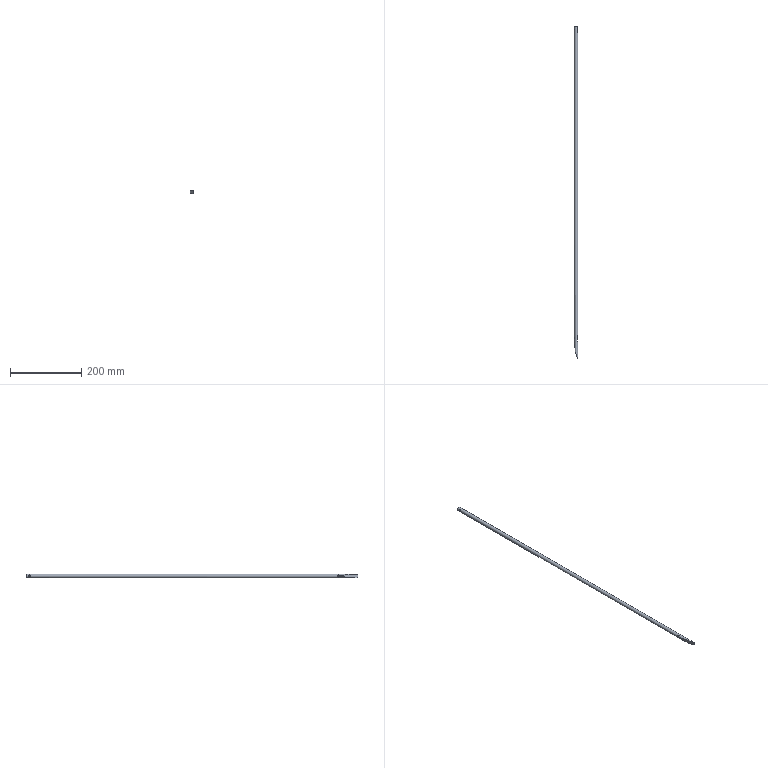Part | NX | 1 solid | 16 faces | box 10 x 930 x 10 mm | volume 71404 mm3 | plane 10 | cylinder 6 | commonest cylinder face diameters 3.4 x2 6 x2 10 x1 380 x1
STEP:
#1=CARTESIAN_POINT('',(-1.,-410.,1.7));
#2=VERTEX_POINT('',#1);
#3=CARTESIAN_POINT('',(-1.,-410.,0.));
#4=DIRECTION('',(-1.,0.,0.));
#5=DIRECTION('',(0.,0.,1.));
#6=AXIS2_PLACEMENT_3D('',#3,#4,#5);
#7=CIRCLE('',#6,1.7);
#8=EDGE_CURVE('',#2,#2,#7,.T.);
#9=ORIENTED_EDGE('',*,*,#8,.T.);
#10=EDGE_LOOP('',(#9));
#11=FACE_BOUND('',#10,.T.);
#12=CARTESIAN_POINT('',(3.,-410.,-1.7));
#13=VERTEX_POINT('',#12);
#14=CARTESIAN_POINT('',(3.,-410.,0.));
#15=DIRECTION('',(1.,0.,0.));
#16=DIRECTION('',(0.,0.,-1.));
#17=AXIS2_PLACEMENT_3D('',#14,#15,#16);
#18=CIRCLE('',#17,1.7);
#19=EDGE_CURVE('',#13,#13,#18,.F.);
#20=ORIENTED_EDGE('',*,*,#19,.F.);
#21=EDGE_LOOP('',(#20));
#22=FACE_BOUND('',#21,.T.);
#23=CARTESIAN_POINT('',(-5.,-410.,0.));
#24=DIRECTION('',(-1.,0.,0.));
#25=DIRECTION('',(0.,0.,1.));
#26=AXIS2_PLACEMENT_3D('',#23,#24,#25);
#27=CYLINDRICAL_SURFACE('',#26,1.7);
#28=ADVANCED_FACE('',(#11,#22),#27,.F.);
#29=CARTESIAN_POINT('',(-1.,455.,1.7));
#30=VERTEX_POINT('',#29);
#31=CARTESIAN_POINT('',(-1.,455.,0.));
#32=DIRECTION('',(-1.,0.,0.));
#33=DIRECTION('',(0.,0.,1.));
#34=AXIS2_PLACEMENT_3D('',#31,#32,#33);
#35=CIRCLE('',#34,1.7);
#36=EDGE_CURVE('',#30,#30,#35,.T.);
#37=ORIENTED_EDGE('',*,*,#36,.T.);
#38=EDGE_LOOP('',(#37));
#39=FACE_BOUND('',#38,.T.);
#40=CARTESIAN_POINT('',(3.,455.,-1.7));
#41=VERTEX_POINT('',#40);
#42=CARTESIAN_POINT('',(3.,455.,0.));
#43=DIRECTION('',(1.,0.,0.));
#44=DIRECTION('',(0.,0.,-1.));
#45=AXIS2_PLACEMENT_3D('',#42,#43,#44);
#46=CIRCLE('',#45,1.7);
#47=EDGE_CURVE('',#41,#41,#46,.F.);
#48=ORIENTED_EDGE('',*,*,#47,.F.);
#49=EDGE_LOOP('',(#48));
#50=FACE_BOUND('',#49,.T.);
#51=CARTESIAN_POINT('',(-5.,455.,0.));
#52=DIRECTION('',(-1.,0.,0.));
#53=DIRECTION('',(0.,0.,1.));
#54=AXIS2_PLACEMENT_3D('',#51,#52,#53);
#55=CYLINDRICAL_SURFACE('',#54,1.7);
#56=ADVANCED_FACE('',(#39,#50),#55,.F.);
#57=CARTESIAN_POINT('',(3.,-402.5,4.));
#58=VERTEX_POINT('',#57);
#59=CARTESIAN_POINT('',(3.,-402.5,-4.));
#60=VERTEX_POINT('',#59);
#61=CARTESIAN_POINT('',(0.,-402.5,0.));
#62=DIRECTION('',(0.,1.,0.));
#63=DIRECTION('',(0.,0.,1.));
#64=AXIS2_PLACEMENT_3D('',#61,#62,#63);
#65=CIRCLE('',#64,5.);
#66=EDGE_CURVE('',#58,#60,#65,.T.);
#67=ORIENTED_EDGE('',*,*,#66,.T.);
#68=CARTESIAN_POINT('',(3.,-417.5,-4.));
#69=VERTEX_POINT('',#68);
#70=CARTESIAN_POINT('',(3.,465.,-4.));
#71=DIRECTION('',(0.,-1.,0.));
#72=VECTOR('',#71,1000.);
#73=LINE('',#70,#72);
#74=EDGE_CURVE('',#69,#60,#73,.F.);
#75=ORIENTED_EDGE('',*,*,#74,.F.);
#76=CARTESIAN_POINT('',(3.,-417.5,4.));
#77=VERTEX_POINT('',#76);
#78=CARTESIAN_POINT('',(0.,-417.5,0.));
#79=DIRECTION('',(0.,-1.,0.));
#80=DIRECTION('',(0.,0.,-1.));
#81=AXIS2_PLACEMENT_3D('',#78,#79,#80);
#82=CIRCLE('',#81,5.);
#83=EDGE_CURVE('',#69,#77,#82,.T.);
#84=ORIENTED_EDGE('',*,*,#83,.T.);
#85=CARTESIAN_POINT('',(3.,465.,4.));
#86=DIRECTION('',(0.,-1.,0.));
#87=VECTOR('',#86,1000.);
#88=LINE('',#85,#87);
#89=EDGE_CURVE('',#58,#77,#88,.T.);
#90=ORIENTED_EDGE('',*,*,#89,.F.);
#91=EDGE_LOOP('',(#67,#75,#84,#90));
#92=FACE_BOUND('',#91,.T.);
#93=CARTESIAN_POINT('',(3.,462.5,4.));
#94=VERTEX_POINT('',#93);
#95=CARTESIAN_POINT('',(3.,462.5,-4.));
#96=VERTEX_POINT('',#95);
#97=CARTESIAN_POINT('',(0.,462.5,0.));
#98=DIRECTION('',(0.,1.,0.));
#99=DIRECTION('',(0.,0.,1.));
#100=AXIS2_PLACEMENT_3D('',#97,#98,#99);
#101=CIRCLE('',#100,5.);
#102=EDGE_CURVE('',#94,#96,#101,.T.);
#103=ORIENTED_EDGE('',*,*,#102,.T.);
#104=CARTESIAN_POINT('',(3.,447.5,-4.));
#105=VERTEX_POINT('',#104);
#106=CARTESIAN_POINT('',(3.,465.,-4.));
#107=DIRECTION('',(0.,-1.,0.));
#108=VECTOR('',#107,1000.);
#109=LINE('',#106,#108);
#110=EDGE_CURVE('',#105,#96,#109,.F.);
#111=ORIENTED_EDGE('',*,*,#110,.F.);
#112=CARTESIAN_POINT('',(3.,447.5,4.));
#113=VERTEX_POINT('',#112);
#114=CARTESIAN_POINT('',(0.,447.5,0.));
#115=DIRECTION('',(0.,-1.,0.));
#116=DIRECTION('',(0.,0.,-1.));
#117=AXIS2_PLACEMENT_3D('',#114,#115,#116);
#118=CIRCLE('',#117,5.);
#119=EDGE_CURVE('',#105,#113,#118,.T.);
#120=ORIENTED_EDGE('',*,*,#119,.T.);
#121=CARTESIAN_POINT('',(3.,465.,4.));
#122=DIRECTION('',(0.,-1.,0.));
#123=VECTOR('',#122,1000.);
#124=LINE('',#121,#123);
#125=EDGE_CURVE('',#94,#113,#124,.T.);
#126=ORIENTED_EDGE('',*,*,#125,.F.);
#127=EDGE_LOOP('',(#103,#111,#120,#126));
#128=FACE_BOUND('',#127,.T.);
#129=CARTESIAN_POINT('',(-4.,455.,3.));
#130=VERTEX_POINT('',#129);
#131=CARTESIAN_POINT('',(-4.552,457.345,2.359));
#132=CARTESIAN_POINT('',(-3.724,454.999,3.321));
#133=CARTESIAN_POINT('',(-4.551,452.658,2.356));
#134=CARTESIAN_POINT('',(-5.223,451.673,0.01399));
#135=CARTESIAN_POINT('',(-4.556,452.651,-2.353));
#136=CARTESIAN_POINT('',(-3.724,454.988,-3.322));
#137=CARTESIAN_POINT('',(-4.549,457.342,-2.36));
#138=CARTESIAN_POINT('',(-5.225,458.328,-0.009275));
#139=CARTESIAN_POINT('',(-4.552,457.345,2.359));
#140=CARTESIAN_POINT('',(-3.724,454.999,3.321));
#141=CARTESIAN_POINT('',(-4.551,452.658,2.356));
#142=B_SPLINE_CURVE_WITH_KNOTS('',3,(#131,#132,#133,#134,#135,#136,#137,#138,#139,#140,#141),.UNSPECIFIED.,.T.,.F.,(1,1,1,1,1,1,1,1,1,1,1,1,1,1,1),(-0.007209,-0.004806,-0.002403,0.,0.002403,0.004806,0.007209,0.009612,0.01202,0.01442,0.01682,0.01922,0.02163,0.02403,0.02643),.UNSPECIFIED.);
#143=EDGE_CURVE('',#130,#130,#142,.T.);
#144=ORIENTED_EDGE('',*,*,#143,.T.);
#145=EDGE_LOOP('',(#144));
#146=FACE_BOUND('',#145,.T.);
#147=CARTESIAN_POINT('',(-4.,-410.,3.));
#148=VERTEX_POINT('',#147);
#149=CARTESIAN_POINT('',(-4.552,-407.655,2.359));
#150=CARTESIAN_POINT('',(-3.724,-410.001,3.321));
#151=CARTESIAN_POINT('',(-4.551,-412.342,2.356));
#152=CARTESIAN_POINT('',(-5.223,-413.327,0.01399));
#153=CARTESIAN_POINT('',(-4.556,-412.349,-2.353));
#154=CARTESIAN_POINT('',(-3.724,-410.012,-3.322));
#155=CARTESIAN_POINT('',(-4.549,-407.658,-2.36));
#156=CARTESIAN_POINT('',(-5.225,-406.672,-0.009275));
#157=CARTESIAN_POINT('',(-4.552,-407.655,2.359));
#158=CARTESIAN_POINT('',(-3.724,-410.001,3.321));
#159=CARTESIAN_POINT('',(-4.551,-412.342,2.356));
#160=B_SPLINE_CURVE_WITH_KNOTS('',3,(#149,#150,#151,#152,#153,#154,#155,#156,#157,#158,#159),.UNSPECIFIED.,.T.,.F.,(1,1,1,1,1,1,1,1,1,1,1,1,1,1,1),(-0.007209,-0.004806,-0.002403,0.,0.002403,0.004806,0.007209,0.009612,0.01202,0.01442,0.01682,0.01922,0.02163,0.02403,0.02643),.UNSPECIFIED.);
#161=EDGE_CURVE('',#148,#148,#160,.T.);
#162=ORIENTED_EDGE('',*,*,#161,.T.);
#163=EDGE_LOOP('',(#162));
#164=FACE_BOUND('',#163,.T.);
#165=CARTESIAN_POINT('',(0.,465.,5.));
#166=VERTEX_POINT('',#165);
#167=CARTESIAN_POINT('',(0.,465.,0.));
#168=DIRECTION('',(0.,1.,0.));
#169=DIRECTION('',(0.,0.,1.));
#170=AXIS2_PLACEMENT_3D('',#167,#168,#169);
#171=CIRCLE('',#170,5.);
#172=EDGE_CURVE('',#166,#166,#171,.T.);
#173=ORIENTED_EDGE('',*,*,#172,.F.);
#174=EDGE_LOOP('',(#173));
#175=FACE_BOUND('',#174,.T.);
#176=CARTESIAN_POINT('',(3.,-465.,4.));
#177=VERTEX_POINT('',#176);
#178=CARTESIAN_POINT('',(3.,-465.,-4.));
#179=VERTEX_POINT('',#178);
#180=CARTESIAN_POINT('',(0.,-465.,0.));
#181=DIRECTION('',(0.,1.,0.));
#182=DIRECTION('',(0.,0.,1.));
#183=AXIS2_PLACEMENT_3D('',#180,#181,#182);
#184=CIRCLE('',#183,5.);
#185=EDGE_CURVE('',#177,#179,#184,.T.);
#186=ORIENTED_EDGE('',*,*,#185,.T.);
#187=CARTESIAN_POINT('',(3.,-465.,-4.));
#188=CARTESIAN_POINT('',(2.387,-462.964,-4.459));
#189=CARTESIAN_POINT('',(1.219,-458.836,-4.942));
#190=CARTESIAN_POINT('',(-0.3371,-452.513,-5.058));
#191=CARTESIAN_POINT('',(-1.662,-446.212,-4.773));
#192=CARTESIAN_POINT('',(-2.767,-439.907,-4.221));
#193=CARTESIAN_POINT('',(-3.507,-434.647,-3.598));
#194=CARTESIAN_POINT('',(-3.993,-430.431,-3.026));
#195=CARTESIAN_POINT('',(-4.305,-427.266,-2.564));
#196=CARTESIAN_POINT('',(-4.563,-424.097,-2.07));
#197=CARTESIAN_POINT('',(-4.734,-421.453,-1.63));
#198=CARTESIAN_POINT('',(-4.844,-419.337,-1.251));
#199=CARTESIAN_POINT('',(-4.902,-418.015,-0.9962));
#200=CARTESIAN_POINT('',(-4.941,-416.958,-0.7702));
#201=CARTESIAN_POINT('',(-4.963,-416.303,-0.6106));
#202=CARTESIAN_POINT('',(-4.979,-415.778,-0.4654));
#203=CARTESIAN_POINT('',(-4.989,-415.41,-0.3229));
#204=CARTESIAN_POINT('',(-4.999,-415.059,-0.2054));
#205=CARTESIAN_POINT('',(-5.001,-414.976,0.08229));
#206=CARTESIAN_POINT('',(-4.994,-415.229,0.2529));
#207=CARTESIAN_POINT('',(-4.986,-415.521,0.3769));
#208=CARTESIAN_POINT('',(-4.972,-416.036,0.5423));
#209=CARTESIAN_POINT('',(-4.951,-416.68,0.7054));
#210=CARTESIAN_POINT('',(-4.923,-417.461,0.8794));
#211=CARTESIAN_POINT('',(-4.881,-418.506,1.093));
#212=CARTESIAN_POINT('',(-4.821,-419.816,1.338));
#213=CARTESIAN_POINT('',(-4.735,-421.389,1.615));
#214=CARTESIAN_POINT('',(-4.636,-422.964,1.881));
#215=CARTESIAN_POINT('',(-4.486,-425.064,2.222));
#216=CARTESIAN_POINT('',(-4.266,-427.691,2.627));
#217=CARTESIAN_POINT('',(-3.949,-430.843,3.084));
#218=CARTESIAN_POINT('',(-3.457,-435.032,3.646));
#219=CARTESIAN_POINT('',(-2.712,-440.248,4.256));
#220=CARTESIAN_POINT('',(-1.61,-446.474,4.79));
#221=CARTESIAN_POINT('',(-0.2985,-452.674,5.057));
#222=CARTESIAN_POINT('',(1.222,-458.839,4.939));
#223=CARTESIAN_POINT('',(2.388,-462.965,4.459));
#224=CARTESIAN_POINT('',(3.,-465.,4.));
#225=B_SPLINE_CURVE_WITH_KNOTS('',3,(#187,#188,#189,#190,#191,#192,#193,#194,#195,#196,#197,#198,#199,#200,#201,#202,#203,#204,#205,#206,#207,#208,#209,#210,#211,#212,#213,#214,#215,#216,#217,#218,#219,#220,#221,#222,#223,#224),.UNSPECIFIED.,.F.,.F.,(4,1,1,1,1,1,1,1,1,1,1,1,1,1,1,1,1,1,1,1,1,1,1,1,1,1,1,1,1,1,1,1,1,1,1,4),(0.,0.006479,0.01296,0.01944,0.02592,0.0324,0.03564,0.03888,0.04212,0.04536,0.04698,0.0486,0.04941,0.05021,0.05062,0.05102,0.05143,0.05163,0.05183,0.05224,0.05264,0.05345,0.05426,0.05507,0.05669,0.05831,0.05993,0.06155,0.06479,0.06803,0.07127,0.07775,0.08423,0.09071,0.09719,0.1037),.UNSPECIFIED.);
#226=EDGE_CURVE('',#179,#177,#225,.T.);
#227=ORIENTED_EDGE('',*,*,#226,.T.);
#228=EDGE_LOOP('',(#186,#227));
#229=FACE_BOUND('',#228,.T.);
#230=CARTESIAN_POINT('',(0.,465.,0.));
#231=DIRECTION('',(0.,-1.,0.));
#232=DIRECTION('',(0.,0.,-1.));
#233=AXIS2_PLACEMENT_3D('',#230,#231,#232);
#234=CYLINDRICAL_SURFACE('',#233,5.);
#235=ADVANCED_FACE('',(#92,#128,#146,#164,#175,#229),#234,.T.);
#236=ORIENTED_EDGE('',*,*,#172,.T.);
#237=EDGE_LOOP('',(#236));
#238=FACE_BOUND('',#237,.T.);
#239=CARTESIAN_POINT('',(0.,465.,0.));
#240=DIRECTION('',(0.,1.,0.));
#241=DIRECTION('',(0.,0.,1.));
#242=AXIS2_PLACEMENT_3D('',#239,#240,#241);
#243=PLANE('',#242);
#244=ADVANCED_FACE('',(#238),#243,.T.);
#245=ORIENTED_EDGE('',*,*,#185,.F.);
#246=CARTESIAN_POINT('',(3.,-465.,-5.));
#247=DIRECTION('',(0.,0.,1.));
#248=VECTOR('',#247,1000.);
#249=LINE('',#246,#248);
#250=EDGE_CURVE('',#177,#179,#249,.F.);
#251=ORIENTED_EDGE('',*,*,#250,.T.);
#252=EDGE_LOOP('',(#245,#251));
#253=FACE_BOUND('',#252,.T.);
#254=CARTESIAN_POINT('',(0.,-465.,0.));
#255=DIRECTION('',(0.,1.,0.));
#256=DIRECTION('',(0.,0.,1.));
#257=AXIS2_PLACEMENT_3D('',#254,#255,#256);
#258=PLANE('',#257);
#259=ADVANCED_FACE('',(#253),#258,.F.);
#260=CARTESIAN_POINT('',(-1.,-410.,3.));
#261=VERTEX_POINT('',#260);
#262=CARTESIAN_POINT('',(-1.,-410.,0.));
#263=DIRECTION('',(-1.,0.,0.));
#264=DIRECTION('',(0.,0.,1.));
#265=AXIS2_PLACEMENT_3D('',#262,#263,#264);
#266=CIRCLE('',#265,3.);
#267=EDGE_CURVE('',#261,#261,#266,.T.);
#268=ORIENTED_EDGE('',*,*,#267,.F.);
#269=EDGE_LOOP('',(#268));
#270=FACE_BOUND('',#269,.T.);
#271=ORIENTED_EDGE('',*,*,#161,.F.);
#272=EDGE_LOOP('',(#271));
#273=FACE_BOUND('',#272,.T.);
#274=CARTESIAN_POINT('',(-5.,-410.,0.));
#275=DIRECTION('',(-1.,0.,0.));
#276=DIRECTION('',(0.,0.,1.));
#277=AXIS2_PLACEMENT_3D('',#274,#275,#276);
#278=CYLINDRICAL_SURFACE('',#277,3.);
#279=ADVANCED_FACE('',(#270,#273),#278,.F.);
#280=ORIENTED_EDGE('',*,*,#8,.F.);
#281=EDGE_LOOP('',(#280));
#282=FACE_BOUND('',#281,.T.);
#283=ORIENTED_EDGE('',*,*,#267,.T.);
#284=EDGE_LOOP('',(#283));
#285=FACE_BOUND('',#284,.T.);
#286=CARTESIAN_POINT('',(-1.,-408.3,0.));
#287=DIRECTION('',(1.,0.,0.));
#288=DIRECTION('',(0.,0.,-1.));
#289=AXIS2_PLACEMENT_3D('',#286,#287,#288);
#290=PLANE('',#289);
#291=ADVANCED_FACE('',(#282,#285),#290,.F.);
#292=CARTESIAN_POINT('',(-1.,455.,3.));
#293=VERTEX_POINT('',#292);
#294=CARTESIAN_POINT('',(-1.,455.,0.));
#295=DIRECTION('',(-1.,0.,0.));
#296=DIRECTION('',(0.,0.,1.));
#297=AXIS2_PLACEMENT_3D('',#294,#295,#296);
#298=CIRCLE('',#297,3.);
#299=EDGE_CURVE('',#293,#293,#298,.T.);
#300=ORIENTED_EDGE('',*,*,#299,.F.);
#301=EDGE_LOOP('',(#300));
#302=FACE_BOUND('',#301,.T.);
#303=ORIENTED_EDGE('',*,*,#143,.F.);
#304=EDGE_LOOP('',(#303));
#305=FACE_BOUND('',#304,.T.);
#306=CARTESIAN_POINT('',(-5.,455.,0.));
#307=DIRECTION('',(-1.,0.,0.));
#308=DIRECTION('',(0.,0.,1.));
#309=AXIS2_PLACEMENT_3D('',#306,#307,#308);
#310=CYLINDRICAL_SURFACE('',#309,3.);
#311=ADVANCED_FACE('',(#302,#305),#310,.F.);
#312=ORIENTED_EDGE('',*,*,#36,.F.);
#313=EDGE_LOOP('',(#312));
#314=FACE_BOUND('',#313,.T.);
#315=ORIENTED_EDGE('',*,*,#299,.T.);
#316=EDGE_LOOP('',(#315));
#317=FACE_BOUND('',#316,.T.);
#318=CARTESIAN_POINT('',(-1.,456.7,0.));
#319=DIRECTION('',(1.,0.,0.));
#320=DIRECTION('',(0.,0.,-1.));
#321=AXIS2_PLACEMENT_3D('',#318,#319,#320);
#322=PLANE('',#321);
#323=ADVANCED_FACE('',(#314,#317),#322,.F.);
#324=CARTESIAN_POINT('',(3.,462.5,-5.));
#325=DIRECTION('',(0.,0.,1.));
#326=VECTOR('',#325,1000.);
#327=LINE('',#324,#326);
#328=EDGE_CURVE('',#96,#94,#327,.T.);
#329=ORIENTED_EDGE('',*,*,#328,.F.);
#330=ORIENTED_EDGE('',*,*,#102,.F.);
#331=EDGE_LOOP('',(#329,#330));
#332=FACE_BOUND('',#331,.T.);
#333=CARTESIAN_POINT('',(3.,462.5,-5.));
#334=DIRECTION('',(0.,1.,0.));
#335=DIRECTION('',(0.,0.,1.));
#336=AXIS2_PLACEMENT_3D('',#333,#334,#335);
#337=PLANE('',#336);
#338=ADVANCED_FACE('',(#332),#337,.F.);
#339=CARTESIAN_POINT('',(3.,447.5,-5.));
#340=DIRECTION('',(0.,0.,-1.));
#341=VECTOR('',#340,1000.);
#342=LINE('',#339,#341);
#343=EDGE_CURVE('',#113,#105,#342,.T.);
#344=ORIENTED_EDGE('',*,*,#343,.F.);
#345=ORIENTED_EDGE('',*,*,#119,.F.);
#346=EDGE_LOOP('',(#344,#345));
#347=FACE_BOUND('',#346,.T.);
#348=CARTESIAN_POINT('',(3.,447.5,-5.));
#349=DIRECTION('',(0.,-1.,0.));
#350=DIRECTION('',(0.,0.,-1.));
#351=AXIS2_PLACEMENT_3D('',#348,#349,#350);
#352=PLANE('',#351);
#353=ADVANCED_FACE('',(#347),#352,.F.);
#354=ORIENTED_EDGE('',*,*,#47,.T.);
#355=EDGE_LOOP('',(#354));
#356=FACE_BOUND('',#355,.T.);
#357=ORIENTED_EDGE('',*,*,#125,.T.);
#358=ORIENTED_EDGE('',*,*,#343,.T.);
#359=ORIENTED_EDGE('',*,*,#110,.T.);
#360=ORIENTED_EDGE('',*,*,#328,.T.);
#361=EDGE_LOOP('',(#357,#358,#359,#360));
#362=FACE_BOUND('',#361,.T.);
#363=CARTESIAN_POINT('',(3.,0.,0.));
#364=DIRECTION('',(1.,0.,0.));
#365=DIRECTION('',(0.,0.,-1.));
#366=AXIS2_PLACEMENT_3D('',#363,#364,#365);
#367=PLANE('',#366);
#368=ADVANCED_FACE('',(#356,#362),#367,.T.);
#369=CARTESIAN_POINT('',(3.,-402.5,-5.));
#370=DIRECTION('',(0.,0.,1.));
#371=VECTOR('',#370,1000.);
#372=LINE('',#369,#371);
#373=EDGE_CURVE('',#60,#58,#372,.T.);
#374=ORIENTED_EDGE('',*,*,#373,.F.);
#375=ORIENTED_EDGE('',*,*,#66,.F.);
#376=EDGE_LOOP('',(#374,#375));
#377=FACE_BOUND('',#376,.T.);
#378=CARTESIAN_POINT('',(3.,-402.5,-5.));
#379=DIRECTION('',(0.,1.,0.));
#380=DIRECTION('',(0.,0.,1.));
#381=AXIS2_PLACEMENT_3D('',#378,#379,#380);
#382=PLANE('',#381);
#383=ADVANCED_FACE('',(#377),#382,.F.);
#384=CARTESIAN_POINT('',(3.,-417.5,-5.));
#385=DIRECTION('',(0.,0.,-1.));
#386=VECTOR('',#385,1000.);
#387=LINE('',#384,#386);
#388=EDGE_CURVE('',#77,#69,#387,.T.);
#389=ORIENTED_EDGE('',*,*,#388,.F.);
#390=ORIENTED_EDGE('',*,*,#83,.F.);
#391=EDGE_LOOP('',(#389,#390));
#392=FACE_BOUND('',#391,.T.);
#393=CARTESIAN_POINT('',(3.,-417.5,-5.));
#394=DIRECTION('',(0.,-1.,0.));
#395=DIRECTION('',(0.,0.,-1.));
#396=AXIS2_PLACEMENT_3D('',#393,#394,#395);
#397=PLANE('',#396);
#398=ADVANCED_FACE('',(#392),#397,.F.);
#399=ORIENTED_EDGE('',*,*,#19,.T.);
#400=EDGE_LOOP('',(#399));
#401=FACE_BOUND('',#400,.T.);
#402=ORIENTED_EDGE('',*,*,#89,.T.);
#403=ORIENTED_EDGE('',*,*,#388,.T.);
#404=ORIENTED_EDGE('',*,*,#74,.T.);
#405=ORIENTED_EDGE('',*,*,#373,.T.);
#406=EDGE_LOOP('',(#402,#403,#404,#405));
#407=FACE_BOUND('',#406,.T.);
#408=CARTESIAN_POINT('',(3.,0.,0.));
#409=DIRECTION('',(1.,0.,0.));
#410=DIRECTION('',(0.,0.,-1.));
#411=AXIS2_PLACEMENT_3D('',#408,#409,#410);
#412=PLANE('',#411);
#413=ADVANCED_FACE('',(#401,#407),#412,.T.);
#414=ORIENTED_EDGE('',*,*,#250,.F.);
#415=ORIENTED_EDGE('',*,*,#226,.F.);
#416=EDGE_LOOP('',(#414,#415));
#417=FACE_BOUND('',#416,.T.);
#418=CARTESIAN_POINT('',(184.941,-410.25,-5.));
#419=DIRECTION('',(0.,0.,1.));
#420=DIRECTION('',(1.,0.,0.));
#421=AXIS2_PLACEMENT_3D('',#418,#419,#420);
#422=CYLINDRICAL_SURFACE('',#421,190.);
#423=ADVANCED_FACE('',(#417),#422,.T.);
#424=CLOSED_SHELL('',(#28,#56,#235,#244,#259,#279,#291,#311,#323,#338,#353,#368,#383,#398,#413,#423));
#425=MANIFOLD_SOLID_BREP('',#424);
#426=(LENGTH_UNIT()NAMED_UNIT(*)SI_UNIT(.MILLI.,.METRE.));
#427=UNCERTAINTY_MEASURE_WITH_UNIT(LENGTH_MEASURE(0.0508),#426,'','');
#428=(NAMED_UNIT(*)PLANE_ANGLE_UNIT()SI_UNIT($,.RADIAN.));
#429=(NAMED_UNIT(*)SI_UNIT($,.STERADIAN.)SOLID_ANGLE_UNIT());
#430=(GEOMETRIC_REPRESENTATION_CONTEXT(3)GLOBAL_UNCERTAINTY_ASSIGNED_CONTEXT((#427))GLOBAL_UNIT_ASSIGNED_CONTEXT((#426,#428,#429))REPRESENTATION_CONTEXT('',''));
#431=ADVANCED_BREP_SHAPE_REPRESENTATION('',(#425),#430);